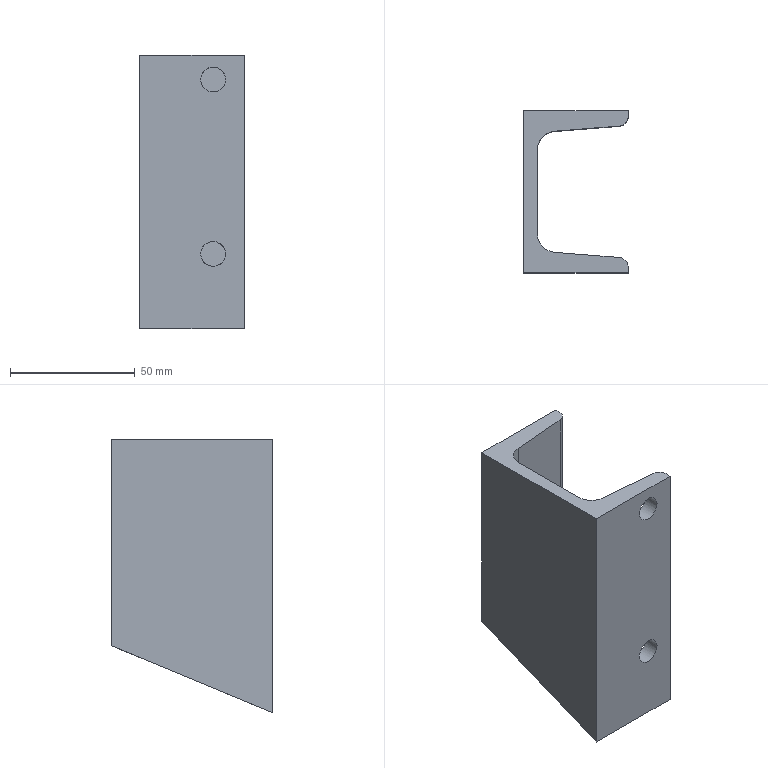Part | STEP file | DIN 1026-1 U 65 1785352380582 | 1 solid | 16 faces | box 42 x 65 x 109.767 mm | volume 85915 mm3 | plane 10 | cylinder 6 | commonest cylinder face diameters 8 x2 10 x2 15 x2
STEP:
#1=CARTESIAN_POINT('',(24.5,-32.5,73.076));
#2=VERTEX_POINT('',#1);
#3=CARTESIAN_POINT('',(29.5,-32.5,73.076));
#4=DIRECTION('',(0.,1.,0.));
#5=DIRECTION('',(1.,0.,0.));
#6=AXIS2_PLACEMENT_3D('',#3,#4,#5);
#7=CIRCLE('',#6,5.);
#8=EDGE_CURVE('',#2,#2,#7,.T.);
#9=ORIENTED_EDGE('',*,*,#8,.F.);
#10=CARTESIAN_POINT('',(24.5,-25.28,73.076));
#11=VERTEX_POINT('',#10);
#12=CARTESIAN_POINT('',(24.5,-32.5,73.076));
#13=DIRECTION('',(0.,1.,0.));
#14=VECTOR('',#13,5.);
#15=LINE('',#12,#14);
#16=EDGE_CURVE('',#2,#11,#15,.T.);
#17=ORIENTED_EDGE('',*,*,#16,.T.);
#18=CARTESIAN_POINT('',(29.5,-25.68,73.076));
#19=DIRECTION('',(-0.07975,-0.9968,0.));
#20=DIRECTION('',(0.9968,-0.07975,0.));
#21=AXIS2_PLACEMENT_3D('',#18,#19,#20);
#22=ELLIPSE('',#21,5.016,5.);
#23=EDGE_CURVE('',#11,#11,#22,.T.);
#24=ORIENTED_EDGE('',*,*,#23,.F.);
#25=ORIENTED_EDGE('',*,*,#16,.F.);
#26=EDGE_LOOP('',(#9,#17,#24,#25));
#27=FACE_OUTER_BOUND('',#26,.T.);
#28=CARTESIAN_POINT('',(29.5,-32.5,73.076));
#29=DIRECTION('',(0.,1.,0.));
#30=DIRECTION('',(1.,0.,0.));
#31=AXIS2_PLACEMENT_3D('',#28,#29,#30);
#32=CYLINDRICAL_SURFACE('',#31,5.);
#33=ADVANCED_FACE('',(#27),#32,.F.);
#34=CARTESIAN_POINT('',(24.5,-32.5,3.076));
#35=VERTEX_POINT('',#34);
#36=CARTESIAN_POINT('',(29.5,-32.5,3.076));
#37=DIRECTION('',(0.,1.,0.));
#38=DIRECTION('',(1.,0.,0.));
#39=AXIS2_PLACEMENT_3D('',#36,#37,#38);
#40=CIRCLE('',#39,5.);
#41=EDGE_CURVE('',#35,#35,#40,.T.);
#42=ORIENTED_EDGE('',*,*,#41,.F.);
#43=CARTESIAN_POINT('',(24.5,-25.28,3.076));
#44=VERTEX_POINT('',#43);
#45=CARTESIAN_POINT('',(24.5,-32.5,3.076));
#46=DIRECTION('',(0.,1.,0.));
#47=VECTOR('',#46,5.);
#48=LINE('',#45,#47);
#49=EDGE_CURVE('',#35,#44,#48,.T.);
#50=ORIENTED_EDGE('',*,*,#49,.T.);
#51=CARTESIAN_POINT('',(29.5,-25.68,3.076));
#52=DIRECTION('',(-0.07975,-0.9968,0.));
#53=DIRECTION('',(0.9968,-0.07975,0.));
#54=AXIS2_PLACEMENT_3D('',#51,#52,#53);
#55=ELLIPSE('',#54,5.016,5.);
#56=EDGE_CURVE('',#44,#44,#55,.T.);
#57=ORIENTED_EDGE('',*,*,#56,.F.);
#58=ORIENTED_EDGE('',*,*,#49,.F.);
#59=EDGE_LOOP('',(#42,#50,#57,#58));
#60=FACE_OUTER_BOUND('',#59,.T.);
#61=CARTESIAN_POINT('',(29.5,-32.5,3.076));
#62=DIRECTION('',(0.,1.,0.));
#63=DIRECTION('',(1.,0.,0.));
#64=AXIS2_PLACEMENT_3D('',#61,#62,#63);
#65=CYLINDRICAL_SURFACE('',#64,5.);
#66=ADVANCED_FACE('',(#60),#65,.F.);
#67=CARTESIAN_POINT('',(12.402,-24.312,-23.532));
#68=VERTEX_POINT('',#67);
#69=CARTESIAN_POINT('',(5.5,-16.836,-20.436));
#70=VERTEX_POINT('',#69);
#71=CARTESIAN_POINT('',(13.,-16.836,-20.436));
#72=DIRECTION('',(0.,0.3827,-0.9239));
#73=DIRECTION('',(0.,-0.9239,-0.3827));
#74=AXIS2_PLACEMENT_3D('',#71,#72,#73);
#75=ELLIPSE('',#74,8.118,7.5);
#76=EDGE_CURVE('',#68,#70,#75,.T.);
#77=ORIENTED_EDGE('',*,*,#76,.F.);
#78=CARTESIAN_POINT('',(38.319,-26.386,-24.391));
#79=VERTEX_POINT('',#78);
#80=CARTESIAN_POINT('',(4.508,-23.681,-23.271));
#81=DIRECTION('',(-0.9963,0.0797,0.03301));
#82=VECTOR('',#81,10.);
#83=LINE('',#80,#82);
#84=EDGE_CURVE('',#79,#68,#83,.T.);
#85=ORIENTED_EDGE('',*,*,#84,.F.);
#86=CARTESIAN_POINT('',(42.,-30.373,-26.043));
#87=VERTEX_POINT('',#86);
#88=CARTESIAN_POINT('',(38.,-30.373,-26.043));
#89=DIRECTION('',(0.,-0.3827,0.9239));
#90=DIRECTION('',(0.,-0.9239,-0.3827));
#91=AXIS2_PLACEMENT_3D('',#88,#89,#90);
#92=ELLIPSE('',#91,4.33,4.);
#93=EDGE_CURVE('',#87,#79,#92,.T.);
#94=ORIENTED_EDGE('',*,*,#93,.F.);
#95=CARTESIAN_POINT('',(42.,-32.5,-26.924));
#96=VERTEX_POINT('',#95);
#97=CARTESIAN_POINT('',(42.,-8.203,-16.86));
#98=DIRECTION('',(0.,0.9239,0.3827));
#99=VECTOR('',#98,10.);
#100=LINE('',#97,#99);
#101=EDGE_CURVE('',#96,#87,#100,.T.);
#102=ORIENTED_EDGE('',*,*,#101,.F.);
#103=CARTESIAN_POINT('',(0.,-32.5,-26.924));
#104=VERTEX_POINT('',#103);
#105=CARTESIAN_POINT('',(31.5,-32.5,-26.924));
#106=DIRECTION('',(-1.,0.,0.));
#107=VECTOR('',#106,10.);
#108=LINE('',#105,#107);
#109=EDGE_CURVE('',#96,#104,#108,.T.);
#110=ORIENTED_EDGE('',*,*,#109,.T.);
#111=CARTESIAN_POINT('',(0.,32.5,0.));
#112=VERTEX_POINT('',#111);
#113=CARTESIAN_POINT('',(0.,4.76,-11.49));
#114=DIRECTION('',(0.,-0.9239,-0.3827));
#115=VECTOR('',#114,10.);
#116=LINE('',#113,#115);
#117=EDGE_CURVE('',#112,#104,#116,.T.);
#118=ORIENTED_EDGE('',*,*,#117,.F.);
#119=CARTESIAN_POINT('',(42.,32.5,0.));
#120=VERTEX_POINT('',#119);
#121=CARTESIAN_POINT('',(0.,32.5,0.));
#122=DIRECTION('',(-1.,0.,0.));
#123=VECTOR('',#122,10.);
#124=LINE('',#121,#123);
#125=EDGE_CURVE('',#120,#112,#124,.T.);
#126=ORIENTED_EDGE('',*,*,#125,.F.);
#127=CARTESIAN_POINT('',(42.,30.373,-0.8811));
#128=VERTEX_POINT('',#127);
#129=CARTESIAN_POINT('',(42.,18.63,-5.745));
#130=DIRECTION('',(0.,0.9239,0.3827));
#131=VECTOR('',#130,10.);
#132=LINE('',#129,#131);
#133=EDGE_CURVE('',#128,#120,#132,.T.);
#134=ORIENTED_EDGE('',*,*,#133,.F.);
#135=CARTESIAN_POINT('',(38.319,26.386,-2.533));
#136=VERTEX_POINT('',#135);
#137=CARTESIAN_POINT('',(38.,30.373,-0.8811));
#138=DIRECTION('',(0.,-0.3827,0.9239));
#139=DIRECTION('',(0.,0.9239,0.3827));
#140=AXIS2_PLACEMENT_3D('',#137,#138,#139);
#141=ELLIPSE('',#140,4.33,4.);
#142=EDGE_CURVE('',#136,#128,#141,.T.);
#143=ORIENTED_EDGE('',*,*,#142,.F.);
#144=CARTESIAN_POINT('',(12.402,24.312,-3.392));
#145=VERTEX_POINT('',#144);
#146=CARTESIAN_POINT('',(18.338,24.787,-3.195));
#147=DIRECTION('',(0.9963,0.0797,0.03301));
#148=VECTOR('',#147,10.);
#149=LINE('',#146,#148);
#150=EDGE_CURVE('',#145,#136,#149,.T.);
#151=ORIENTED_EDGE('',*,*,#150,.F.);
#152=CARTESIAN_POINT('',(5.5,16.836,-6.488));
#153=VERTEX_POINT('',#152);
#154=CARTESIAN_POINT('',(13.,16.836,-6.488));
#155=DIRECTION('',(0.,0.3827,-0.9239));
#156=DIRECTION('',(0.,0.9239,0.3827));
#157=AXIS2_PLACEMENT_3D('',#154,#155,#156);
#158=ELLIPSE('',#157,8.118,7.5);
#159=EDGE_CURVE('',#153,#145,#158,.T.);
#160=ORIENTED_EDGE('',*,*,#159,.F.);
#161=CARTESIAN_POINT('',(5.5,4.76,-11.49));
#162=DIRECTION('',(0.,0.9239,0.3827));
#163=VECTOR('',#162,10.);
#164=LINE('',#161,#163);
#165=EDGE_CURVE('',#70,#153,#164,.T.);
#166=ORIENTED_EDGE('',*,*,#165,.F.);
#167=EDGE_LOOP('',(#77,#85,#94,#102,#110,#118,#126,#134,#143,#151,#160,#166));
#168=FACE_OUTER_BOUND('',#167,.T.);
#169=CARTESIAN_POINT('',(0.,4.76,-11.49));
#170=DIRECTION('',(0.,-0.3827,0.9239));
#171=DIRECTION('',(1.,0.,0.));
#172=AXIS2_PLACEMENT_3D('',#169,#170,#171);
#173=PLANE('',#172);
#174=ADVANCED_FACE('',(#168),#173,.F.);
#175=ORIENTED_EDGE('',*,*,#125,.T.);
#176=CARTESIAN_POINT('',(0.,32.5,82.843));
#177=VERTEX_POINT('',#176);
#178=CARTESIAN_POINT('',(0.,32.5,0.));
#179=DIRECTION('',(0.,0.,-1.));
#180=VECTOR('',#179,10.);
#181=LINE('',#178,#180);
#182=EDGE_CURVE('',#177,#112,#181,.T.);
#183=ORIENTED_EDGE('',*,*,#182,.F.);
#184=CARTESIAN_POINT('',(42.,32.5,82.843));
#185=VERTEX_POINT('',#184);
#186=CARTESIAN_POINT('',(10.5,32.5,82.843));
#187=DIRECTION('',(1.,0.,0.));
#188=VECTOR('',#187,10.);
#189=LINE('',#186,#188);
#190=EDGE_CURVE('',#177,#185,#189,.T.);
#191=ORIENTED_EDGE('',*,*,#190,.T.);
#192=CARTESIAN_POINT('',(42.,32.5,0.));
#193=DIRECTION('',(0.,0.,-1.));
#194=VECTOR('',#193,10.);
#195=LINE('',#192,#194);
#196=EDGE_CURVE('',#185,#120,#195,.T.);
#197=ORIENTED_EDGE('',*,*,#196,.T.);
#198=EDGE_LOOP('',(#175,#183,#191,#197));
#199=FACE_OUTER_BOUND('',#198,.T.);
#200=CARTESIAN_POINT('',(0.,32.5,0.));
#201=DIRECTION('',(0.,1.,0.));
#202=DIRECTION('',(0.,0.,1.));
#203=AXIS2_PLACEMENT_3D('',#200,#201,#202);
#204=PLANE('',#203);
#205=ADVANCED_FACE('',(#199),#204,.T.);
#206=ORIENTED_EDGE('',*,*,#117,.T.);
#207=CARTESIAN_POINT('',(0.,-32.5,82.843));
#208=VERTEX_POINT('',#207);
#209=CARTESIAN_POINT('',(0.,-32.5,0.));
#210=DIRECTION('',(0.,0.,-1.));
#211=VECTOR('',#210,10.);
#212=LINE('',#209,#211);
#213=EDGE_CURVE('',#208,#104,#212,.T.);
#214=ORIENTED_EDGE('',*,*,#213,.F.);
#215=CARTESIAN_POINT('',(0.,0.,82.843));
#216=DIRECTION('',(0.,1.,0.));
#217=VECTOR('',#216,10.);
#218=LINE('',#215,#217);
#219=EDGE_CURVE('',#208,#177,#218,.T.);
#220=ORIENTED_EDGE('',*,*,#219,.T.);
#221=ORIENTED_EDGE('',*,*,#182,.T.);
#222=EDGE_LOOP('',(#206,#214,#220,#221));
#223=FACE_OUTER_BOUND('',#222,.T.);
#224=CARTESIAN_POINT('',(0.,0.,0.));
#225=DIRECTION('',(-1.,0.,0.));
#226=DIRECTION('',(0.,0.,1.));
#227=AXIS2_PLACEMENT_3D('',#224,#225,#226);
#228=PLANE('',#227);
#229=ADVANCED_FACE('',(#223),#228,.T.);
#230=ORIENTED_EDGE('',*,*,#101,.T.);
#231=CARTESIAN_POINT('',(42.,-30.373,82.843));
#232=VERTEX_POINT('',#231);
#233=CARTESIAN_POINT('',(42.,-30.373,0.));
#234=DIRECTION('',(0.,0.,-1.));
#235=VECTOR('',#234,10.);
#236=LINE('',#233,#235);
#237=EDGE_CURVE('',#232,#87,#236,.T.);
#238=ORIENTED_EDGE('',*,*,#237,.F.);
#239=CARTESIAN_POINT('',(42.,-32.5,82.843));
#240=VERTEX_POINT('',#239);
#241=CARTESIAN_POINT('',(42.,-15.186,82.843));
#242=DIRECTION('',(0.,-1.,0.));
#243=VECTOR('',#242,10.);
#244=LINE('',#241,#243);
#245=EDGE_CURVE('',#232,#240,#244,.T.);
#246=ORIENTED_EDGE('',*,*,#245,.T.);
#247=CARTESIAN_POINT('',(42.,-32.5,0.));
#248=DIRECTION('',(0.,0.,-1.));
#249=VECTOR('',#248,10.);
#250=LINE('',#247,#249);
#251=EDGE_CURVE('',#240,#96,#250,.T.);
#252=ORIENTED_EDGE('',*,*,#251,.T.);
#253=EDGE_LOOP('',(#230,#238,#246,#252));
#254=FACE_OUTER_BOUND('',#253,.T.);
#255=CARTESIAN_POINT('',(42.,-30.373,0.));
#256=DIRECTION('',(1.,0.,0.));
#257=DIRECTION('',(0.,0.,-1.));
#258=AXIS2_PLACEMENT_3D('',#255,#256,#257);
#259=PLANE('',#258);
#260=ADVANCED_FACE('',(#254),#259,.T.);
#261=ORIENTED_EDGE('',*,*,#93,.T.);
#262=CARTESIAN_POINT('',(38.319,-26.386,82.843));
#263=VERTEX_POINT('',#262);
#264=CARTESIAN_POINT('',(38.319,-26.386,0.));
#265=DIRECTION('',(0.,0.,-1.));
#266=VECTOR('',#265,10.);
#267=LINE('',#264,#266);
#268=EDGE_CURVE('',#263,#79,#267,.T.);
#269=ORIENTED_EDGE('',*,*,#268,.F.);
#270=CARTESIAN_POINT('',(38.,-30.373,82.843));
#271=DIRECTION('',(0.,0.,-1.));
#272=DIRECTION('',(-1.,0.,0.));
#273=AXIS2_PLACEMENT_3D('',#270,#271,#272);
#274=CIRCLE('',#273,4.);
#275=EDGE_CURVE('',#263,#232,#274,.T.);
#276=ORIENTED_EDGE('',*,*,#275,.T.);
#277=ORIENTED_EDGE('',*,*,#237,.T.);
#278=EDGE_LOOP('',(#261,#269,#276,#277));
#279=FACE_OUTER_BOUND('',#278,.T.);
#280=CARTESIAN_POINT('',(38.,-30.373,0.));
#281=DIRECTION('',(0.,0.,1.));
#282=DIRECTION('',(-1.,0.,0.));
#283=AXIS2_PLACEMENT_3D('',#280,#281,#282);
#284=CYLINDRICAL_SURFACE('',#283,4.);
#285=ADVANCED_FACE('',(#279),#284,.T.);
#286=ORIENTED_EDGE('',*,*,#84,.T.);
#287=CARTESIAN_POINT('',(12.402,-24.312,82.843));
#288=VERTEX_POINT('',#287);
#289=CARTESIAN_POINT('',(12.402,-24.312,0.));
#290=DIRECTION('',(0.,0.,-1.));
#291=VECTOR('',#290,10.);
#292=LINE('',#289,#291);
#293=EDGE_CURVE('',#288,#68,#292,.T.);
#294=ORIENTED_EDGE('',*,*,#293,.F.);
#295=CARTESIAN_POINT('',(15.707,-24.577,82.843));
#296=DIRECTION('',(0.9968,-0.07975,0.));
#297=VECTOR('',#296,10.);
#298=LINE('',#295,#297);
#299=EDGE_CURVE('',#288,#263,#298,.T.);
#300=ORIENTED_EDGE('',*,*,#299,.T.);
#301=ORIENTED_EDGE('',*,*,#268,.T.);
#302=EDGE_LOOP('',(#286,#294,#300,#301));
#303=FACE_OUTER_BOUND('',#302,.T.);
#304=ORIENTED_EDGE('',*,*,#23,.T.);
#305=EDGE_LOOP('',(#304));
#306=FACE_BOUND('',#305,.T.);
#307=ORIENTED_EDGE('',*,*,#56,.T.);
#308=EDGE_LOOP('',(#307));
#309=FACE_BOUND('',#308,.T.);
#310=CARTESIAN_POINT('',(12.402,-24.312,0.));
#311=DIRECTION('',(0.07975,0.9968,0.));
#312=DIRECTION('',(0.,0.,1.));
#313=AXIS2_PLACEMENT_3D('',#310,#311,#312);
#314=PLANE('',#313);
#315=ADVANCED_FACE('',(#303,#306,#309),#314,.T.);
#316=ORIENTED_EDGE('',*,*,#76,.T.);
#317=CARTESIAN_POINT('',(5.5,-16.836,82.843));
#318=VERTEX_POINT('',#317);
#319=CARTESIAN_POINT('',(5.5,-16.836,0.));
#320=DIRECTION('',(0.,0.,-1.));
#321=VECTOR('',#320,10.);
#322=LINE('',#319,#321);
#323=EDGE_CURVE('',#318,#70,#322,.T.);
#324=ORIENTED_EDGE('',*,*,#323,.F.);
#325=CARTESIAN_POINT('',(13.,-16.836,82.843));
#326=DIRECTION('',(0.,0.,1.));
#327=DIRECTION('',(-1.,0.,0.));
#328=AXIS2_PLACEMENT_3D('',#325,#326,#327);
#329=CIRCLE('',#328,7.5);
#330=EDGE_CURVE('',#318,#288,#329,.T.);
#331=ORIENTED_EDGE('',*,*,#330,.T.);
#332=ORIENTED_EDGE('',*,*,#293,.T.);
#333=EDGE_LOOP('',(#316,#324,#331,#332));
#334=FACE_OUTER_BOUND('',#333,.T.);
#335=CARTESIAN_POINT('',(13.,-16.836,0.));
#336=DIRECTION('',(0.,0.,1.));
#337=DIRECTION('',(-1.,0.,0.));
#338=AXIS2_PLACEMENT_3D('',#335,#336,#337);
#339=CYLINDRICAL_SURFACE('',#338,7.5);
#340=ADVANCED_FACE('',(#334),#339,.F.);
#341=CARTESIAN_POINT('',(31.5,-32.5,82.843));
#342=DIRECTION('',(-1.,0.,0.));
#343=VECTOR('',#342,10.);
#344=LINE('',#341,#343);
#345=EDGE_CURVE('',#240,#208,#344,.T.);
#346=ORIENTED_EDGE('',*,*,#345,.T.);
#347=ORIENTED_EDGE('',*,*,#213,.T.);
#348=ORIENTED_EDGE('',*,*,#109,.F.);
#349=ORIENTED_EDGE('',*,*,#251,.F.);
#350=EDGE_LOOP('',(#346,#347,#348,#349));
#351=FACE_OUTER_BOUND('',#350,.T.);
#352=ORIENTED_EDGE('',*,*,#8,.T.);
#353=EDGE_LOOP('',(#352));
#354=FACE_BOUND('',#353,.T.);
#355=ORIENTED_EDGE('',*,*,#41,.T.);
#356=EDGE_LOOP('',(#355));
#357=FACE_BOUND('',#356,.T.);
#358=CARTESIAN_POINT('',(42.,-32.5,0.));
#359=DIRECTION('',(0.,-1.,0.));
#360=DIRECTION('',(0.,0.,-1.));
#361=AXIS2_PLACEMENT_3D('',#358,#359,#360);
#362=PLANE('',#361);
#363=ADVANCED_FACE('',(#351,#354,#357),#362,.T.);
#364=ORIENTED_EDGE('',*,*,#133,.T.);
#365=ORIENTED_EDGE('',*,*,#196,.F.);
#366=CARTESIAN_POINT('',(42.,30.373,82.843));
#367=VERTEX_POINT('',#366);
#368=CARTESIAN_POINT('',(42.,16.25,82.843));
#369=DIRECTION('',(0.,-1.,0.));
#370=VECTOR('',#369,10.);
#371=LINE('',#368,#370);
#372=EDGE_CURVE('',#185,#367,#371,.T.);
#373=ORIENTED_EDGE('',*,*,#372,.T.);
#374=CARTESIAN_POINT('',(42.,30.373,0.));
#375=DIRECTION('',(0.,0.,-1.));
#376=VECTOR('',#375,10.);
#377=LINE('',#374,#376);
#378=EDGE_CURVE('',#367,#128,#377,.T.);
#379=ORIENTED_EDGE('',*,*,#378,.T.);
#380=EDGE_LOOP('',(#364,#365,#373,#379));
#381=FACE_OUTER_BOUND('',#380,.T.);
#382=CARTESIAN_POINT('',(42.,32.5,0.));
#383=DIRECTION('',(1.,0.,0.));
#384=DIRECTION('',(0.,0.,-1.));
#385=AXIS2_PLACEMENT_3D('',#382,#383,#384);
#386=PLANE('',#385);
#387=ADVANCED_FACE('',(#381),#386,.T.);
#388=ORIENTED_EDGE('',*,*,#142,.T.);
#389=ORIENTED_EDGE('',*,*,#378,.F.);
#390=CARTESIAN_POINT('',(38.319,26.386,82.843));
#391=VERTEX_POINT('',#390);
#392=CARTESIAN_POINT('',(38.,30.373,82.843));
#393=DIRECTION('',(0.,0.,-1.));
#394=DIRECTION('',(-0.07975,0.9968,0.));
#395=AXIS2_PLACEMENT_3D('',#392,#393,#394);
#396=CIRCLE('',#395,4.);
#397=EDGE_CURVE('',#367,#391,#396,.T.);
#398=ORIENTED_EDGE('',*,*,#397,.T.);
#399=CARTESIAN_POINT('',(38.319,26.386,0.));
#400=DIRECTION('',(0.,0.,-1.));
#401=VECTOR('',#400,10.);
#402=LINE('',#399,#401);
#403=EDGE_CURVE('',#391,#136,#402,.T.);
#404=ORIENTED_EDGE('',*,*,#403,.T.);
#405=EDGE_LOOP('',(#388,#389,#398,#404));
#406=FACE_OUTER_BOUND('',#405,.T.);
#407=CARTESIAN_POINT('',(38.,30.373,0.));
#408=DIRECTION('',(0.,0.,1.));
#409=DIRECTION('',(-0.07975,0.9968,0.));
#410=AXIS2_PLACEMENT_3D('',#407,#408,#409);
#411=CYLINDRICAL_SURFACE('',#410,4.);
#412=ADVANCED_FACE('',(#406),#411,.T.);
#413=ORIENTED_EDGE('',*,*,#150,.T.);
#414=ORIENTED_EDGE('',*,*,#403,.F.);
#415=CARTESIAN_POINT('',(12.402,24.312,82.843));
#416=VERTEX_POINT('',#415);
#417=CARTESIAN_POINT('',(28.666,25.613,82.843));
#418=DIRECTION('',(-0.9968,-0.07975,0.));
#419=VECTOR('',#418,10.);
#420=LINE('',#417,#419);
#421=EDGE_CURVE('',#391,#416,#420,.T.);
#422=ORIENTED_EDGE('',*,*,#421,.T.);
#423=CARTESIAN_POINT('',(12.402,24.312,0.));
#424=DIRECTION('',(0.,0.,-1.));
#425=VECTOR('',#424,10.);
#426=LINE('',#423,#425);
#427=EDGE_CURVE('',#416,#145,#426,.T.);
#428=ORIENTED_EDGE('',*,*,#427,.T.);
#429=EDGE_LOOP('',(#413,#414,#422,#428));
#430=FACE_OUTER_BOUND('',#429,.T.);
#431=CARTESIAN_POINT('',(38.319,26.386,0.));
#432=DIRECTION('',(0.07975,-0.9968,0.));
#433=DIRECTION('',(0.,0.,-1.));
#434=AXIS2_PLACEMENT_3D('',#431,#432,#433);
#435=PLANE('',#434);
#436=ADVANCED_FACE('',(#430),#435,.T.);
#437=ORIENTED_EDGE('',*,*,#159,.T.);
#438=ORIENTED_EDGE('',*,*,#427,.F.);
#439=CARTESIAN_POINT('',(5.5,16.836,82.843));
#440=VERTEX_POINT('',#439);
#441=CARTESIAN_POINT('',(13.,16.836,82.843));
#442=DIRECTION('',(0.,0.,1.));
#443=DIRECTION('',(-0.07975,0.9968,0.));
#444=AXIS2_PLACEMENT_3D('',#441,#442,#443);
#445=CIRCLE('',#444,7.5);
#446=EDGE_CURVE('',#416,#440,#445,.T.);
#447=ORIENTED_EDGE('',*,*,#446,.T.);
#448=CARTESIAN_POINT('',(5.5,16.836,0.));
#449=DIRECTION('',(0.,0.,-1.));
#450=VECTOR('',#449,10.);
#451=LINE('',#448,#450);
#452=EDGE_CURVE('',#440,#153,#451,.T.);
#453=ORIENTED_EDGE('',*,*,#452,.T.);
#454=EDGE_LOOP('',(#437,#438,#447,#453));
#455=FACE_OUTER_BOUND('',#454,.T.);
#456=CARTESIAN_POINT('',(13.,16.836,0.));
#457=DIRECTION('',(0.,0.,1.));
#458=DIRECTION('',(-0.07975,0.9968,0.));
#459=AXIS2_PLACEMENT_3D('',#456,#457,#458);
#460=CYLINDRICAL_SURFACE('',#459,7.5);
#461=ADVANCED_FACE('',(#455),#460,.F.);
#462=ORIENTED_EDGE('',*,*,#165,.T.);
#463=ORIENTED_EDGE('',*,*,#452,.F.);
#464=CARTESIAN_POINT('',(5.5,0.,82.843));
#465=DIRECTION('',(0.,-1.,0.));
#466=VECTOR('',#465,10.);
#467=LINE('',#464,#466);
#468=EDGE_CURVE('',#440,#318,#467,.T.);
#469=ORIENTED_EDGE('',*,*,#468,.T.);
#470=ORIENTED_EDGE('',*,*,#323,.T.);
#471=EDGE_LOOP('',(#462,#463,#469,#470));
#472=FACE_OUTER_BOUND('',#471,.T.);
#473=CARTESIAN_POINT('',(5.5,0.,0.));
#474=DIRECTION('',(1.,0.,0.));
#475=DIRECTION('',(0.,0.,-1.));
#476=AXIS2_PLACEMENT_3D('',#473,#474,#475);
#477=PLANE('',#476);
#478=ADVANCED_FACE('',(#472),#477,.T.);
#479=ORIENTED_EDGE('',*,*,#190,.F.);
#480=ORIENTED_EDGE('',*,*,#219,.F.);
#481=ORIENTED_EDGE('',*,*,#345,.F.);
#482=ORIENTED_EDGE('',*,*,#245,.F.);
#483=ORIENTED_EDGE('',*,*,#275,.F.);
#484=ORIENTED_EDGE('',*,*,#299,.F.);
#485=ORIENTED_EDGE('',*,*,#330,.F.);
#486=ORIENTED_EDGE('',*,*,#468,.F.);
#487=ORIENTED_EDGE('',*,*,#446,.F.);
#488=ORIENTED_EDGE('',*,*,#421,.F.);
#489=ORIENTED_EDGE('',*,*,#397,.F.);
#490=ORIENTED_EDGE('',*,*,#372,.F.);
#491=EDGE_LOOP('',(#479,#480,#481,#482,#483,#484,#485,#486,#487,#488,#489,#490));
#492=FACE_OUTER_BOUND('',#491,.T.);
#493=CARTESIAN_POINT('',(21.,0.,82.843));
#494=DIRECTION('',(0.,0.,1.));
#495=DIRECTION('',(1.,0.,0.));
#496=AXIS2_PLACEMENT_3D('',#493,#494,#495);
#497=PLANE('',#496);
#498=ADVANCED_FACE('',(#492),#497,.T.);
#499=CLOSED_SHELL('',(#33,#66,#174,#205,#229,#260,#285,#315,#340,#363,#387,#412,#436,#461,#478,#498));
#500=MANIFOLD_SOLID_BREP('',#499);
#501=(LENGTH_UNIT()NAMED_UNIT(*)SI_UNIT(.MILLI.,.METRE.));
#502=UNCERTAINTY_MEASURE_WITH_UNIT(LENGTH_MEASURE(0.01),#501,'','');
#503=(NAMED_UNIT(*)PLANE_ANGLE_UNIT()SI_UNIT($,.RADIAN.));
#504=(NAMED_UNIT(*)SI_UNIT($,.STERADIAN.)SOLID_ANGLE_UNIT());
#505=(GEOMETRIC_REPRESENTATION_CONTEXT(3)GLOBAL_UNCERTAINTY_ASSIGNED_CONTEXT((#502))GLOBAL_UNIT_ASSIGNED_CONTEXT((#501,#503,#504))REPRESENTATION_CONTEXT('',''));
#506=ADVANCED_BREP_SHAPE_REPRESENTATION('',(#500),#505);